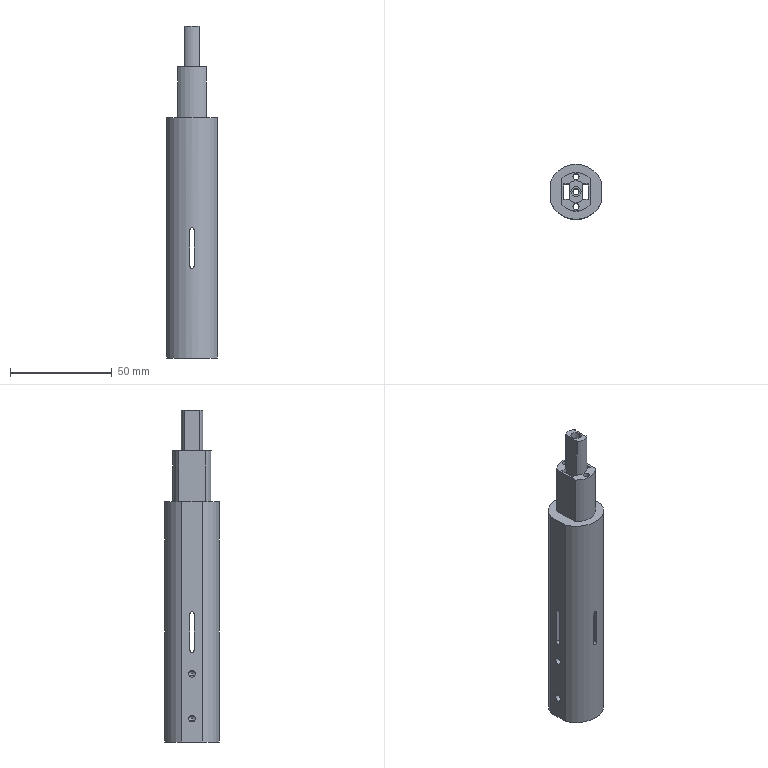Part | STEP file | magnetic tile slingshot detection base seat | 1 solid | 115 faces | box 25 x 27 x 163 mm | volume 57664 mm3 | cylinder 64 | plane 39 | cone 12 | commonest cylinder face diameters 2 x20 3.3 x16 5 x8 3 x6 6.2 x4 6.8 x4